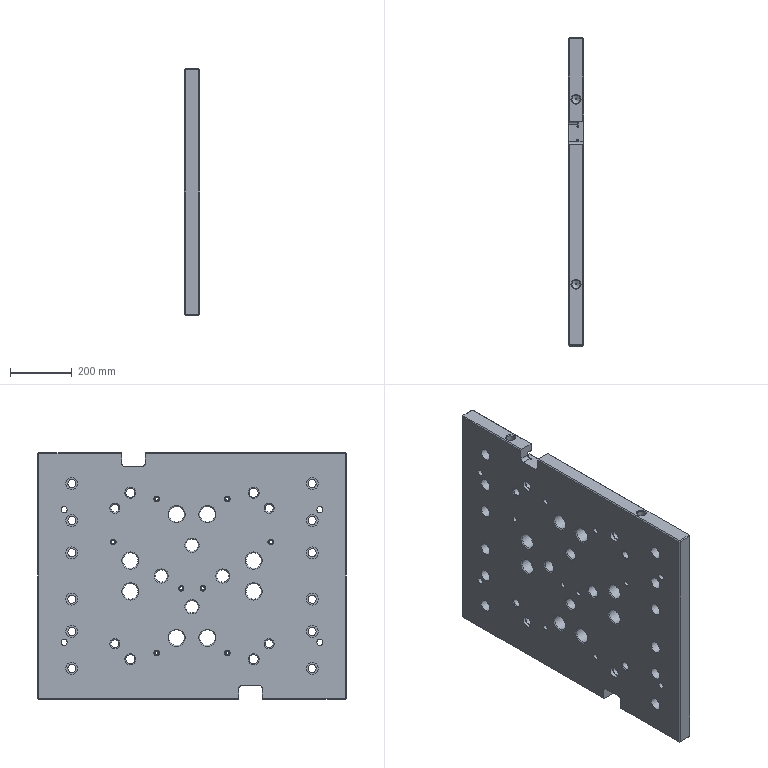Part | STEP file | solid 71 | 1 solid | 712 faces | box 50 x 1000 x 800 mm | volume 37110850 mm3 | plane 383 | cylinder 198 | cone 128 | torus 3 | commonest cylinder face diameters 15 x70 4.2 x17 8 x15 26 x12 39 x12 11 x8